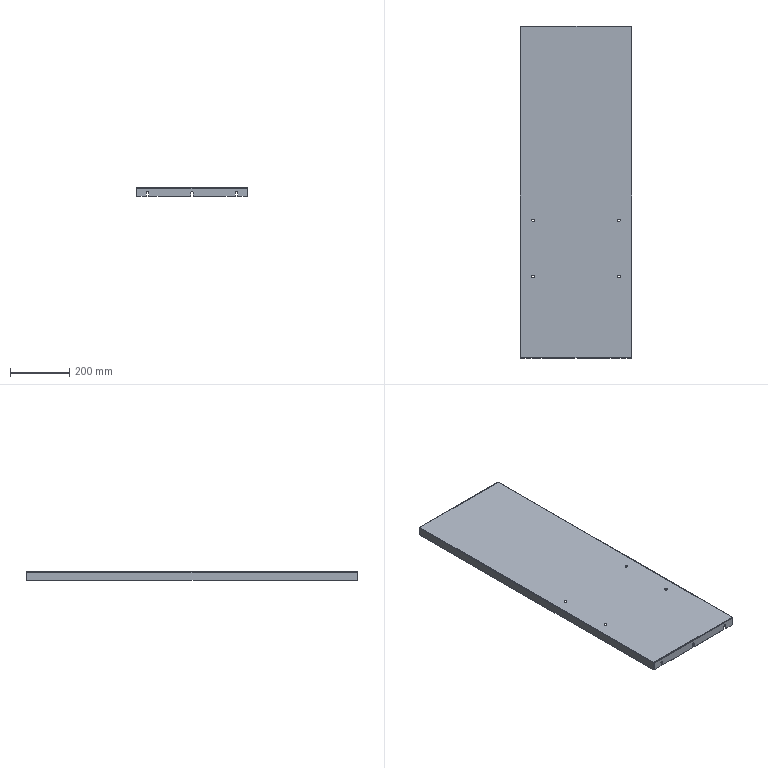Part | 1 solid | 70 faces | box 378 x 1121 x 30 mm | volume 608262 mm3 | plane 40 | cylinder 22 | spline 8 | commonest cylinder face diameters 8.6 x8 8.2 x6 1.473 x4 3.873 x4